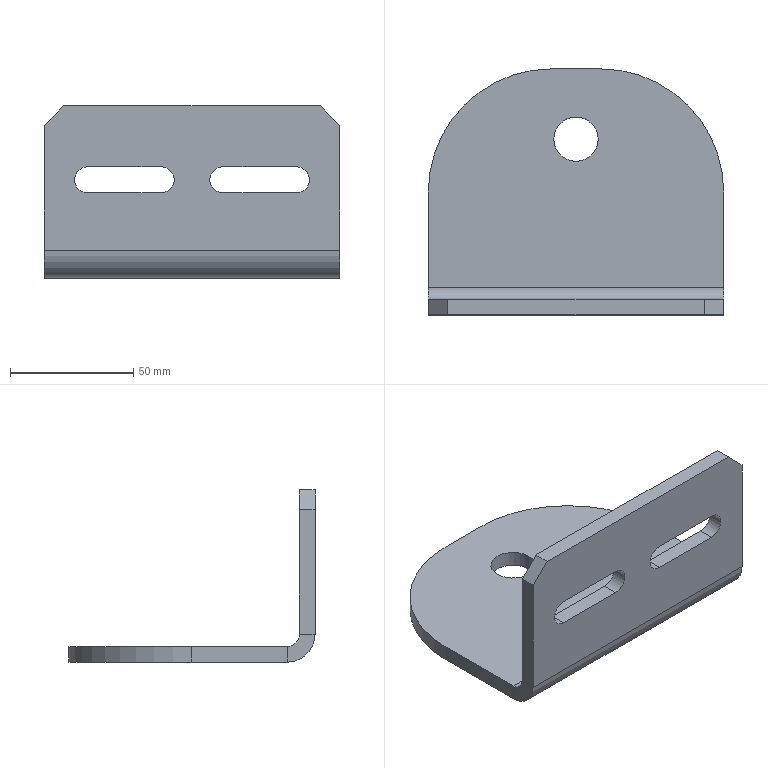Part | STEP file | BASE POLEA_SHEET METAL | 1 solid | 28 faces | box 120 x 100 x 70 mm | volume 108092 mm3 | plane 18 | cylinder 10 | commonest cylinder face diameters 10.5 x4 18 x2 100 x2 10 x1 22.7 x1
STEP:
#1=CARTESIAN_POINT('',(-9.,71.5,0.));
#2=VERTEX_POINT('',#1);
#3=CARTESIAN_POINT('',(9.,71.5,0.));
#4=VERTEX_POINT('',#3);
#5=CARTESIAN_POINT('',(0.,71.5,0.));
#6=DIRECTION('',(0.,0.,1.));
#7=DIRECTION('',(1.,0.,0.));
#8=AXIS2_PLACEMENT_3D('',#5,#6,#7);
#9=CIRCLE('',#8,9.);
#10=EDGE_CURVE('',#2,#4,#9,.T.);
#11=ORIENTED_EDGE('',*,*,#10,.F.);
#12=CARTESIAN_POINT('',(-9.,71.5,6.35));
#13=VERTEX_POINT('',#12);
#14=CARTESIAN_POINT('',(-9.,71.5,-3.65));
#15=DIRECTION('',(0.,0.,1.));
#16=VECTOR('',#15,1000.);
#17=LINE('',#14,#16);
#18=EDGE_CURVE('',#2,#13,#17,.T.);
#19=ORIENTED_EDGE('',*,*,#18,.T.);
#20=CARTESIAN_POINT('',(9.,71.5,6.35));
#21=VERTEX_POINT('',#20);
#22=CARTESIAN_POINT('',(0.,71.5,6.35));
#23=DIRECTION('',(0.,0.,1.));
#24=DIRECTION('',(1.,0.,0.));
#25=AXIS2_PLACEMENT_3D('',#22,#23,#24);
#26=CIRCLE('',#25,9.);
#27=EDGE_CURVE('',#13,#21,#26,.T.);
#28=ORIENTED_EDGE('',*,*,#27,.T.);
#29=CARTESIAN_POINT('',(9.,71.5,-3.65));
#30=DIRECTION('',(0.,0.,1.));
#31=VECTOR('',#30,1000.);
#32=LINE('',#29,#31);
#33=EDGE_CURVE('',#4,#21,#32,.T.);
#34=ORIENTED_EDGE('',*,*,#33,.F.);
#35=EDGE_LOOP('',(#11,#19,#28,#34));
#36=FACE_OUTER_BOUND('',#35,.T.);
#37=CARTESIAN_POINT('',(0.,71.5,-3.65));
#38=DIRECTION('',(0.,0.,1.));
#39=DIRECTION('',(1.,0.,0.));
#40=AXIS2_PLACEMENT_3D('',#37,#38,#39);
#41=CYLINDRICAL_SURFACE('',#40,9.);
#42=ADVANCED_FACE('',(#36),#41,.F.);
#43=CARTESIAN_POINT('',(60.,0.,11.35));
#44=VERTEX_POINT('',#43);
#45=CARTESIAN_POINT('',(60.,6.35,11.35));
#46=VERTEX_POINT('',#45);
#47=CARTESIAN_POINT('',(60.,0.,11.35));
#48=DIRECTION('',(0.,1.,0.));
#49=VECTOR('',#48,1000.);
#50=LINE('',#47,#49);
#51=EDGE_CURVE('',#44,#46,#50,.T.);
#52=ORIENTED_EDGE('',*,*,#51,.F.);
#53=CARTESIAN_POINT('',(60.,11.35,0.));
#54=VERTEX_POINT('',#53);
#55=CARTESIAN_POINT('',(60.,11.35,11.35));
#56=DIRECTION('',(1.,0.,0.));
#57=DIRECTION('',(0.,0.,1.));
#58=AXIS2_PLACEMENT_3D('',#55,#56,#57);
#59=CIRCLE('',#58,11.35);
#60=EDGE_CURVE('',#44,#54,#59,.T.);
#61=ORIENTED_EDGE('',*,*,#60,.T.);
#62=CARTESIAN_POINT('',(60.,11.35,6.35));
#63=VERTEX_POINT('',#62);
#64=CARTESIAN_POINT('',(60.,11.35,6.35));
#65=DIRECTION('',(0.,0.,-1.));
#66=VECTOR('',#65,1000.);
#67=LINE('',#64,#66);
#68=EDGE_CURVE('',#63,#54,#67,.T.);
#69=ORIENTED_EDGE('',*,*,#68,.F.);
#70=CARTESIAN_POINT('',(60.,11.35,11.35));
#71=DIRECTION('',(1.,0.,0.));
#72=DIRECTION('',(0.,0.,-1.));
#73=AXIS2_PLACEMENT_3D('',#70,#71,#72);
#74=CIRCLE('',#73,5.);
#75=EDGE_CURVE('',#46,#63,#74,.T.);
#76=ORIENTED_EDGE('',*,*,#75,.F.);
#77=EDGE_LOOP('',(#52,#61,#69,#76));
#78=FACE_OUTER_BOUND('',#77,.T.);
#79=CARTESIAN_POINT('',(60.,0.,11.35));
#80=DIRECTION('',(1.,0.,0.));
#81=DIRECTION('',(0.,0.,-1.));
#82=AXIS2_PLACEMENT_3D('',#79,#80,#81);
#83=PLANE('',#82);
#84=ADVANCED_FACE('',(#78),#83,.T.);
#85=CARTESIAN_POINT('',(60.,6.35,62.));
#86=VERTEX_POINT('',#85);
#87=CARTESIAN_POINT('',(60.,6.35,70.));
#88=DIRECTION('',(0.,0.,-1.));
#89=VECTOR('',#88,1000.);
#90=LINE('',#87,#89);
#91=EDGE_CURVE('',#86,#46,#90,.T.);
#92=ORIENTED_EDGE('',*,*,#91,.F.);
#93=CARTESIAN_POINT('',(60.,0.,62.));
#94=VERTEX_POINT('',#93);
#95=CARTESIAN_POINT('',(60.,11.35,62.));
#96=DIRECTION('',(0.,-1.,0.));
#97=VECTOR('',#96,1000.);
#98=LINE('',#95,#97);
#99=EDGE_CURVE('',#86,#94,#98,.T.);
#100=ORIENTED_EDGE('',*,*,#99,.T.);
#101=CARTESIAN_POINT('',(60.,0.,70.));
#102=DIRECTION('',(0.,0.,-1.));
#103=VECTOR('',#102,1000.);
#104=LINE('',#101,#103);
#105=EDGE_CURVE('',#94,#44,#104,.T.);
#106=ORIENTED_EDGE('',*,*,#105,.T.);
#107=ORIENTED_EDGE('',*,*,#51,.T.);
#108=EDGE_LOOP('',(#92,#100,#106,#107));
#109=FACE_OUTER_BOUND('',#108,.T.);
#110=CARTESIAN_POINT('',(60.,11.35,6.35));
#111=DIRECTION('',(1.,0.,0.));
#112=DIRECTION('',(0.,0.,-1.));
#113=AXIS2_PLACEMENT_3D('',#110,#111,#112);
#114=PLANE('',#113);
#115=ADVANCED_FACE('',(#109),#114,.T.);
#116=CARTESIAN_POINT('',(-60.,11.35,0.));
#117=VERTEX_POINT('',#116);
#118=CARTESIAN_POINT('',(-60.,11.35,6.35));
#119=VERTEX_POINT('',#118);
#120=CARTESIAN_POINT('',(-60.,11.35,0.));
#121=DIRECTION('',(0.,0.,1.));
#122=VECTOR('',#121,1000.);
#123=LINE('',#120,#122);
#124=EDGE_CURVE('',#117,#119,#123,.T.);
#125=ORIENTED_EDGE('',*,*,#124,.F.);
#126=CARTESIAN_POINT('',(-60.,0.,11.35));
#127=VERTEX_POINT('',#126);
#128=CARTESIAN_POINT('',(-60.,11.35,11.35));
#129=DIRECTION('',(1.,0.,0.));
#130=DIRECTION('',(0.,0.,1.));
#131=AXIS2_PLACEMENT_3D('',#128,#129,#130);
#132=CIRCLE('',#131,11.35);
#133=EDGE_CURVE('',#127,#117,#132,.T.);
#134=ORIENTED_EDGE('',*,*,#133,.F.);
#135=CARTESIAN_POINT('',(-60.,6.35,11.35));
#136=VERTEX_POINT('',#135);
#137=CARTESIAN_POINT('',(-60.,6.35,11.35));
#138=DIRECTION('',(0.,-1.,0.));
#139=VECTOR('',#138,1000.);
#140=LINE('',#137,#139);
#141=EDGE_CURVE('',#136,#127,#140,.T.);
#142=ORIENTED_EDGE('',*,*,#141,.F.);
#143=CARTESIAN_POINT('',(-60.,11.35,11.35));
#144=DIRECTION('',(1.,0.,0.));
#145=DIRECTION('',(0.,0.,-1.));
#146=AXIS2_PLACEMENT_3D('',#143,#144,#145);
#147=CIRCLE('',#146,5.);
#148=EDGE_CURVE('',#136,#119,#147,.T.);
#149=ORIENTED_EDGE('',*,*,#148,.T.);
#150=EDGE_LOOP('',(#125,#134,#142,#149));
#151=FACE_OUTER_BOUND('',#150,.T.);
#152=CARTESIAN_POINT('',(-60.,11.35,0.));
#153=DIRECTION('',(-1.,0.,0.));
#154=DIRECTION('',(0.,0.,1.));
#155=AXIS2_PLACEMENT_3D('',#152,#153,#154);
#156=PLANE('',#155);
#157=ADVANCED_FACE('',(#151),#156,.T.);
#158=CARTESIAN_POINT('',(-60.,50.,6.35));
#159=VERTEX_POINT('',#158);
#160=CARTESIAN_POINT('',(-60.,0.,6.35));
#161=DIRECTION('',(0.,1.,0.));
#162=VECTOR('',#161,1000.);
#163=LINE('',#160,#162);
#164=EDGE_CURVE('',#119,#159,#163,.T.);
#165=ORIENTED_EDGE('',*,*,#164,.T.);
#166=CARTESIAN_POINT('',(-60.,50.,0.));
#167=VERTEX_POINT('',#166);
#168=CARTESIAN_POINT('',(-60.,50.,11.35));
#169=DIRECTION('',(0.,0.,-1.));
#170=VECTOR('',#169,1000.);
#171=LINE('',#168,#170);
#172=EDGE_CURVE('',#159,#167,#171,.T.);
#173=ORIENTED_EDGE('',*,*,#172,.T.);
#174=CARTESIAN_POINT('',(-60.,0.,0.));
#175=DIRECTION('',(0.,1.,0.));
#176=VECTOR('',#175,1000.);
#177=LINE('',#174,#176);
#178=EDGE_CURVE('',#117,#167,#177,.T.);
#179=ORIENTED_EDGE('',*,*,#178,.F.);
#180=ORIENTED_EDGE('',*,*,#124,.T.);
#181=EDGE_LOOP('',(#165,#173,#179,#180));
#182=FACE_OUTER_BOUND('',#181,.T.);
#183=CARTESIAN_POINT('',(-60.,6.35,11.35));
#184=DIRECTION('',(-1.,0.,0.));
#185=DIRECTION('',(0.,0.,1.));
#186=AXIS2_PLACEMENT_3D('',#183,#184,#185);
#187=PLANE('',#186);
#188=ADVANCED_FACE('',(#182),#187,.T.);
#189=CARTESIAN_POINT('',(0.,71.5,0.));
#190=DIRECTION('',(0.,0.,1.));
#191=DIRECTION('',(1.,0.,0.));
#192=AXIS2_PLACEMENT_3D('',#189,#190,#191);
#193=CIRCLE('',#192,9.);
#194=EDGE_CURVE('',#4,#2,#193,.T.);
#195=ORIENTED_EDGE('',*,*,#194,.T.);
#196=ORIENTED_EDGE('',*,*,#10,.T.);
#197=EDGE_LOOP('',(#195,#196));
#198=FACE_BOUND('',#197,.T.);
#199=ORIENTED_EDGE('',*,*,#178,.T.);
#200=CARTESIAN_POINT('',(-10.,100.,0.));
#201=VERTEX_POINT('',#200);
#202=CARTESIAN_POINT('',(-10.,50.,0.));
#203=DIRECTION('',(0.,0.,-1.));
#204=DIRECTION('',(1.,0.,0.));
#205=AXIS2_PLACEMENT_3D('',#202,#203,#204);
#206=CIRCLE('',#205,50.);
#207=EDGE_CURVE('',#167,#201,#206,.T.);
#208=ORIENTED_EDGE('',*,*,#207,.T.);
#209=CARTESIAN_POINT('',(10.,100.,0.));
#210=VERTEX_POINT('',#209);
#211=CARTESIAN_POINT('',(60.,100.,0.));
#212=DIRECTION('',(-1.,0.,0.));
#213=VECTOR('',#212,1000.);
#214=LINE('',#211,#213);
#215=EDGE_CURVE('',#210,#201,#214,.T.);
#216=ORIENTED_EDGE('',*,*,#215,.F.);
#217=CARTESIAN_POINT('',(60.,50.,0.));
#218=VERTEX_POINT('',#217);
#219=CARTESIAN_POINT('',(10.,50.,0.));
#220=DIRECTION('',(0.,0.,-1.));
#221=DIRECTION('',(1.,0.,0.));
#222=AXIS2_PLACEMENT_3D('',#219,#220,#221);
#223=CIRCLE('',#222,50.);
#224=EDGE_CURVE('',#210,#218,#223,.T.);
#225=ORIENTED_EDGE('',*,*,#224,.T.);
#226=CARTESIAN_POINT('',(60.,0.,0.));
#227=DIRECTION('',(0.,1.,0.));
#228=VECTOR('',#227,1000.);
#229=LINE('',#226,#228);
#230=EDGE_CURVE('',#54,#218,#229,.T.);
#231=ORIENTED_EDGE('',*,*,#230,.F.);
#232=CARTESIAN_POINT('',(60.,11.35,0.));
#233=DIRECTION('',(-1.,0.,0.));
#234=VECTOR('',#233,1000.);
#235=LINE('',#232,#234);
#236=EDGE_CURVE('',#54,#117,#235,.T.);
#237=ORIENTED_EDGE('',*,*,#236,.T.);
#238=EDGE_LOOP('',(#199,#208,#216,#225,#231,#237));
#239=FACE_OUTER_BOUND('',#238,.T.);
#240=CARTESIAN_POINT('',(60.,0.,0.));
#241=DIRECTION('',(0.,0.,1.));
#242=DIRECTION('',(1.,0.,0.));
#243=AXIS2_PLACEMENT_3D('',#240,#241,#242);
#244=PLANE('',#243);
#245=ADVANCED_FACE('',(#198,#239),#244,.F.);
#246=ORIENTED_EDGE('',*,*,#215,.T.);
#247=CARTESIAN_POINT('',(-10.,100.,6.35));
#248=VERTEX_POINT('',#247);
#249=CARTESIAN_POINT('',(-10.,100.,6.35));
#250=DIRECTION('',(0.,0.,1.));
#251=VECTOR('',#250,1000.);
#252=LINE('',#249,#251);
#253=EDGE_CURVE('',#201,#248,#252,.T.);
#254=ORIENTED_EDGE('',*,*,#253,.T.);
#255=CARTESIAN_POINT('',(10.,100.,6.35));
#256=VERTEX_POINT('',#255);
#257=CARTESIAN_POINT('',(60.,100.,6.35));
#258=DIRECTION('',(-1.,0.,0.));
#259=VECTOR('',#258,1000.);
#260=LINE('',#257,#259);
#261=EDGE_CURVE('',#256,#248,#260,.T.);
#262=ORIENTED_EDGE('',*,*,#261,.F.);
#263=CARTESIAN_POINT('',(10.,100.,6.35));
#264=DIRECTION('',(0.,0.,-1.));
#265=VECTOR('',#264,1000.);
#266=LINE('',#263,#265);
#267=EDGE_CURVE('',#256,#210,#266,.T.);
#268=ORIENTED_EDGE('',*,*,#267,.T.);
#269=EDGE_LOOP('',(#246,#254,#262,#268));
#270=FACE_OUTER_BOUND('',#269,.T.);
#271=CARTESIAN_POINT('',(60.,100.,6.35));
#272=DIRECTION('',(0.,1.,0.));
#273=DIRECTION('',(0.,0.,1.));
#274=AXIS2_PLACEMENT_3D('',#271,#272,#273);
#275=PLANE('',#274);
#276=ADVANCED_FACE('',(#270),#275,.T.);
#277=CARTESIAN_POINT('',(0.,71.5,6.35));
#278=DIRECTION('',(0.,0.,1.));
#279=DIRECTION('',(1.,0.,0.));
#280=AXIS2_PLACEMENT_3D('',#277,#278,#279);
#281=CIRCLE('',#280,9.);
#282=EDGE_CURVE('',#21,#13,#281,.T.);
#283=ORIENTED_EDGE('',*,*,#282,.F.);
#284=ORIENTED_EDGE('',*,*,#27,.F.);
#285=EDGE_LOOP('',(#283,#284));
#286=FACE_BOUND('',#285,.T.);
#287=ORIENTED_EDGE('',*,*,#261,.T.);
#288=CARTESIAN_POINT('',(-10.,50.,6.35));
#289=DIRECTION('',(0.,0.,1.));
#290=DIRECTION('',(1.,0.,0.));
#291=AXIS2_PLACEMENT_3D('',#288,#289,#290);
#292=CIRCLE('',#291,50.);
#293=EDGE_CURVE('',#248,#159,#292,.T.);
#294=ORIENTED_EDGE('',*,*,#293,.T.);
#295=ORIENTED_EDGE('',*,*,#164,.F.);
#296=CARTESIAN_POINT('',(60.,11.35,6.35));
#297=DIRECTION('',(-1.,0.,0.));
#298=VECTOR('',#297,1000.);
#299=LINE('',#296,#298);
#300=EDGE_CURVE('',#63,#119,#299,.T.);
#301=ORIENTED_EDGE('',*,*,#300,.F.);
#302=CARTESIAN_POINT('',(60.,50.,6.35));
#303=VERTEX_POINT('',#302);
#304=CARTESIAN_POINT('',(60.,0.,6.35));
#305=DIRECTION('',(0.,1.,0.));
#306=VECTOR('',#305,1000.);
#307=LINE('',#304,#306);
#308=EDGE_CURVE('',#63,#303,#307,.T.);
#309=ORIENTED_EDGE('',*,*,#308,.T.);
#310=CARTESIAN_POINT('',(10.,50.,6.35));
#311=DIRECTION('',(0.,0.,1.));
#312=DIRECTION('',(1.,0.,0.));
#313=AXIS2_PLACEMENT_3D('',#310,#311,#312);
#314=CIRCLE('',#313,50.);
#315=EDGE_CURVE('',#303,#256,#314,.T.);
#316=ORIENTED_EDGE('',*,*,#315,.T.);
#317=EDGE_LOOP('',(#287,#294,#295,#301,#309,#316));
#318=FACE_OUTER_BOUND('',#317,.T.);
#319=CARTESIAN_POINT('',(60.,0.,6.35));
#320=DIRECTION('',(0.,0.,1.));
#321=DIRECTION('',(1.,0.,0.));
#322=AXIS2_PLACEMENT_3D('',#319,#320,#321);
#323=PLANE('',#322);
#324=ADVANCED_FACE('',(#286,#318),#323,.T.);
#325=ORIENTED_EDGE('',*,*,#148,.F.);
#326=CARTESIAN_POINT('',(60.,6.35,11.35));
#327=DIRECTION('',(-1.,0.,0.));
#328=VECTOR('',#327,1000.);
#329=LINE('',#326,#328);
#330=EDGE_CURVE('',#46,#136,#329,.T.);
#331=ORIENTED_EDGE('',*,*,#330,.F.);
#332=ORIENTED_EDGE('',*,*,#75,.T.);
#333=ORIENTED_EDGE('',*,*,#300,.T.);
#334=EDGE_LOOP('',(#325,#331,#332,#333));
#335=FACE_OUTER_BOUND('',#334,.T.);
#336=CARTESIAN_POINT('',(60.,11.35,11.35));
#337=DIRECTION('',(-1.,0.,0.));
#338=DIRECTION('',(0.,0.,1.));
#339=AXIS2_PLACEMENT_3D('',#336,#337,#338);
#340=CYLINDRICAL_SURFACE('',#339,5.);
#341=ADVANCED_FACE('',(#335),#340,.F.);
#342=CARTESIAN_POINT('',(-42.5,6.35,34.75));
#343=VERTEX_POINT('',#342);
#344=CARTESIAN_POINT('',(-42.5,6.35,45.25));
#345=VERTEX_POINT('',#344);
#346=CARTESIAN_POINT('',(-42.5,6.35,40.));
#347=DIRECTION('',(0.,1.,0.));
#348=DIRECTION('',(0.,0.,1.));
#349=AXIS2_PLACEMENT_3D('',#346,#347,#348);
#350=CIRCLE('',#349,5.25);
#351=EDGE_CURVE('',#343,#345,#350,.T.);
#352=ORIENTED_EDGE('',*,*,#351,.F.);
#353=CARTESIAN_POINT('',(-12.5,6.35,34.75));
#354=VERTEX_POINT('',#353);
#355=CARTESIAN_POINT('',(-42.5,6.35,34.75));
#356=DIRECTION('',(-1.,0.,0.));
#357=VECTOR('',#356,1000.);
#358=LINE('',#355,#357);
#359=EDGE_CURVE('',#354,#343,#358,.T.);
#360=ORIENTED_EDGE('',*,*,#359,.F.);
#361=CARTESIAN_POINT('',(-12.5,6.35,45.25));
#362=VERTEX_POINT('',#361);
#363=CARTESIAN_POINT('',(-12.5,6.35,40.));
#364=DIRECTION('',(0.,1.,0.));
#365=DIRECTION('',(0.,0.,1.));
#366=AXIS2_PLACEMENT_3D('',#363,#364,#365);
#367=CIRCLE('',#366,5.25);
#368=EDGE_CURVE('',#362,#354,#367,.T.);
#369=ORIENTED_EDGE('',*,*,#368,.F.);
#370=CARTESIAN_POINT('',(-42.5,6.35,45.25));
#371=DIRECTION('',(1.,0.,0.));
#372=VECTOR('',#371,1000.);
#373=LINE('',#370,#372);
#374=EDGE_CURVE('',#345,#362,#373,.T.);
#375=ORIENTED_EDGE('',*,*,#374,.F.);
#376=EDGE_LOOP('',(#352,#360,#369,#375));
#377=FACE_BOUND('',#376,.T.);
#378=CARTESIAN_POINT('',(42.5,6.35,45.25));
#379=VERTEX_POINT('',#378);
#380=CARTESIAN_POINT('',(42.5,6.35,34.75));
#381=VERTEX_POINT('',#380);
#382=CARTESIAN_POINT('',(42.5,6.35,40.));
#383=DIRECTION('',(0.,1.,0.));
#384=DIRECTION('',(0.,0.,-1.));
#385=AXIS2_PLACEMENT_3D('',#382,#383,#384);
#386=CIRCLE('',#385,5.25);
#387=EDGE_CURVE('',#379,#381,#386,.T.);
#388=ORIENTED_EDGE('',*,*,#387,.F.);
#389=CARTESIAN_POINT('',(12.5,6.35,45.25));
#390=VERTEX_POINT('',#389);
#391=CARTESIAN_POINT('',(42.5,6.35,45.25));
#392=DIRECTION('',(1.,0.,0.));
#393=VECTOR('',#392,1000.);
#394=LINE('',#391,#393);
#395=EDGE_CURVE('',#390,#379,#394,.T.);
#396=ORIENTED_EDGE('',*,*,#395,.F.);
#397=CARTESIAN_POINT('',(12.5,6.35,34.75));
#398=VERTEX_POINT('',#397);
#399=CARTESIAN_POINT('',(12.5,6.35,40.));
#400=DIRECTION('',(0.,1.,0.));
#401=DIRECTION('',(0.,0.,-1.));
#402=AXIS2_PLACEMENT_3D('',#399,#400,#401);
#403=CIRCLE('',#402,5.25);
#404=EDGE_CURVE('',#398,#390,#403,.T.);
#405=ORIENTED_EDGE('',*,*,#404,.F.);
#406=CARTESIAN_POINT('',(42.5,6.35,34.75));
#407=DIRECTION('',(-1.,0.,0.));
#408=VECTOR('',#407,1000.);
#409=LINE('',#406,#408);
#410=EDGE_CURVE('',#381,#398,#409,.T.);
#411=ORIENTED_EDGE('',*,*,#410,.F.);
#412=EDGE_LOOP('',(#388,#396,#405,#411));
#413=FACE_BOUND('',#412,.T.);
#414=CARTESIAN_POINT('',(-60.,6.35,62.));
#415=VERTEX_POINT('',#414);
#416=CARTESIAN_POINT('',(-60.,6.35,70.));
#417=DIRECTION('',(0.,0.,-1.));
#418=VECTOR('',#417,1000.);
#419=LINE('',#416,#418);
#420=EDGE_CURVE('',#415,#136,#419,.T.);
#421=ORIENTED_EDGE('',*,*,#420,.F.);
#422=CARTESIAN_POINT('',(-52.,6.35,70.));
#423=VERTEX_POINT('',#422);
#424=CARTESIAN_POINT('',(4.,6.35,126.));
#425=DIRECTION('',(0.7071,0.,0.7071));
#426=VECTOR('',#425,1000.);
#427=LINE('',#424,#426);
#428=EDGE_CURVE('',#415,#423,#427,.T.);
#429=ORIENTED_EDGE('',*,*,#428,.T.);
#430=CARTESIAN_POINT('',(52.,6.35,70.));
#431=VERTEX_POINT('',#430);
#432=CARTESIAN_POINT('',(60.,6.35,70.));
#433=DIRECTION('',(-1.,0.,0.));
#434=VECTOR('',#433,1000.);
#435=LINE('',#432,#434);
#436=EDGE_CURVE('',#431,#423,#435,.T.);
#437=ORIENTED_EDGE('',*,*,#436,.F.);
#438=CARTESIAN_POINT('',(56.,6.35,66.));
#439=DIRECTION('',(0.7071,0.,-0.7071));
#440=VECTOR('',#439,1000.);
#441=LINE('',#438,#440);
#442=EDGE_CURVE('',#431,#86,#441,.T.);
#443=ORIENTED_EDGE('',*,*,#442,.T.);
#444=ORIENTED_EDGE('',*,*,#91,.T.);
#445=ORIENTED_EDGE('',*,*,#330,.T.);
#446=EDGE_LOOP('',(#421,#429,#437,#443,#444,#445));
#447=FACE_OUTER_BOUND('',#446,.T.);
#448=CARTESIAN_POINT('',(60.,6.35,70.));
#449=DIRECTION('',(0.,1.,0.));
#450=DIRECTION('',(0.,0.,1.));
#451=AXIS2_PLACEMENT_3D('',#448,#449,#450);
#452=PLANE('',#451);
#453=ADVANCED_FACE('',(#377,#413,#447),#452,.T.);
#454=ORIENTED_EDGE('',*,*,#436,.T.);
#455=CARTESIAN_POINT('',(-52.,0.,70.));
#456=VERTEX_POINT('',#455);
#457=CARTESIAN_POINT('',(-52.,0.,70.));
#458=DIRECTION('',(0.,-1.,0.));
#459=VECTOR('',#458,1000.);
#460=LINE('',#457,#459);
#461=EDGE_CURVE('',#423,#456,#460,.T.);
#462=ORIENTED_EDGE('',*,*,#461,.T.);
#463=CARTESIAN_POINT('',(52.,0.,70.));
#464=VERTEX_POINT('',#463);
#465=CARTESIAN_POINT('',(60.,0.,70.));
#466=DIRECTION('',(-1.,0.,0.));
#467=VECTOR('',#466,1000.);
#468=LINE('',#465,#467);
#469=EDGE_CURVE('',#464,#456,#468,.T.);
#470=ORIENTED_EDGE('',*,*,#469,.F.);
#471=CARTESIAN_POINT('',(52.,0.,70.));
#472=DIRECTION('',(0.,1.,0.));
#473=VECTOR('',#472,1000.);
#474=LINE('',#471,#473);
#475=EDGE_CURVE('',#464,#431,#474,.T.);
#476=ORIENTED_EDGE('',*,*,#475,.T.);
#477=EDGE_LOOP('',(#454,#462,#470,#476));
#478=FACE_OUTER_BOUND('',#477,.T.);
#479=CARTESIAN_POINT('',(60.,0.,70.));
#480=DIRECTION('',(0.,0.,1.));
#481=DIRECTION('',(1.,0.,0.));
#482=AXIS2_PLACEMENT_3D('',#479,#480,#481);
#483=PLANE('',#482);
#484=ADVANCED_FACE('',(#478),#483,.T.);
#485=CARTESIAN_POINT('',(-12.5,0.,34.75));
#486=VERTEX_POINT('',#485);
#487=CARTESIAN_POINT('',(-42.5,0.,34.75));
#488=VERTEX_POINT('',#487);
#489=CARTESIAN_POINT('',(-42.5,0.,34.75));
#490=DIRECTION('',(-1.,0.,0.));
#491=VECTOR('',#490,1000.);
#492=LINE('',#489,#491);
#493=EDGE_CURVE('',#486,#488,#492,.T.);
#494=ORIENTED_EDGE('',*,*,#493,.T.);
#495=CARTESIAN_POINT('',(-42.5,0.,45.25));
#496=VERTEX_POINT('',#495);
#497=CARTESIAN_POINT('',(-42.5,0.,40.));
#498=DIRECTION('',(0.,1.,0.));
#499=DIRECTION('',(0.,0.,1.));
#500=AXIS2_PLACEMENT_3D('',#497,#498,#499);
#501=CIRCLE('',#500,5.25);
#502=EDGE_CURVE('',#488,#496,#501,.T.);
#503=ORIENTED_EDGE('',*,*,#502,.T.);
#504=CARTESIAN_POINT('',(-12.5,0.,45.25));
#505=VERTEX_POINT('',#504);
#506=CARTESIAN_POINT('',(-42.5,0.,45.25));
#507=DIRECTION('',(1.,0.,0.));
#508=VECTOR('',#507,1000.);
#509=LINE('',#506,#508);
#510=EDGE_CURVE('',#496,#505,#509,.T.);
#511=ORIENTED_EDGE('',*,*,#510,.T.);
#512=CARTESIAN_POINT('',(-12.5,0.,40.));
#513=DIRECTION('',(0.,1.,0.));
#514=DIRECTION('',(0.,0.,1.));
#515=AXIS2_PLACEMENT_3D('',#512,#513,#514);
#516=CIRCLE('',#515,5.25);
#517=EDGE_CURVE('',#505,#486,#516,.T.);
#518=ORIENTED_EDGE('',*,*,#517,.T.);
#519=EDGE_LOOP('',(#494,#503,#511,#518));
#520=FACE_BOUND('',#519,.T.);
#521=CARTESIAN_POINT('',(12.5,0.,45.25));
#522=VERTEX_POINT('',#521);
#523=CARTESIAN_POINT('',(42.5,0.,45.25));
#524=VERTEX_POINT('',#523);
#525=CARTESIAN_POINT('',(42.5,0.,45.25));
#526=DIRECTION('',(1.,0.,0.));
#527=VECTOR('',#526,1000.);
#528=LINE('',#525,#527);
#529=EDGE_CURVE('',#522,#524,#528,.T.);
#530=ORIENTED_EDGE('',*,*,#529,.T.);
#531=CARTESIAN_POINT('',(42.5,0.,34.75));
#532=VERTEX_POINT('',#531);
#533=CARTESIAN_POINT('',(42.5,0.,40.));
#534=DIRECTION('',(0.,1.,0.));
#535=DIRECTION('',(0.,0.,-1.));
#536=AXIS2_PLACEMENT_3D('',#533,#534,#535);
#537=CIRCLE('',#536,5.25);
#538=EDGE_CURVE('',#524,#532,#537,.T.);
#539=ORIENTED_EDGE('',*,*,#538,.T.);
#540=CARTESIAN_POINT('',(12.5,0.,34.75));
#541=VERTEX_POINT('',#540);
#542=CARTESIAN_POINT('',(42.5,0.,34.75));
#543=DIRECTION('',(-1.,0.,0.));
#544=VECTOR('',#543,1000.);
#545=LINE('',#542,#544);
#546=EDGE_CURVE('',#532,#541,#545,.T.);
#547=ORIENTED_EDGE('',*,*,#546,.T.);
#548=CARTESIAN_POINT('',(12.5,0.,40.));
#549=DIRECTION('',(0.,1.,0.));
#550=DIRECTION('',(0.,0.,-1.));
#551=AXIS2_PLACEMENT_3D('',#548,#549,#550);
#552=CIRCLE('',#551,5.25);
#553=EDGE_CURVE('',#541,#522,#552,.T.);
#554=ORIENTED_EDGE('',*,*,#553,.T.);
#555=EDGE_LOOP('',(#530,#539,#547,#554));
#556=FACE_BOUND('',#555,.T.);
#557=ORIENTED_EDGE('',*,*,#469,.T.);
#558=CARTESIAN_POINT('',(-60.,0.,62.));
#559=VERTEX_POINT('',#558);
#560=CARTESIAN_POINT('',(-60.,0.,62.));
#561=DIRECTION('',(-0.7071,0.,-0.7071));
#562=VECTOR('',#561,1000.);
#563=LINE('',#560,#562);
#564=EDGE_CURVE('',#456,#559,#563,.T.);
#565=ORIENTED_EDGE('',*,*,#564,.T.);
#566=CARTESIAN_POINT('',(-60.,0.,70.));
#567=DIRECTION('',(0.,0.,-1.));
#568=VECTOR('',#567,1000.);
#569=LINE('',#566,#568);
#570=EDGE_CURVE('',#559,#127,#569,.T.);
#571=ORIENTED_EDGE('',*,*,#570,.T.);
#572=CARTESIAN_POINT('',(60.,0.,11.35));
#573=DIRECTION('',(-1.,0.,0.));
#574=VECTOR('',#573,1000.);
#575=LINE('',#572,#574);
#576=EDGE_CURVE('',#44,#127,#575,.T.);
#577=ORIENTED_EDGE('',*,*,#576,.F.);
#578=ORIENTED_EDGE('',*,*,#105,.F.);
#579=CARTESIAN_POINT('',(52.,0.,70.));
#580=DIRECTION('',(-0.7071,0.,0.7071));
#581=VECTOR('',#580,1000.);
#582=LINE('',#579,#581);
#583=EDGE_CURVE('',#94,#464,#582,.T.);
#584=ORIENTED_EDGE('',*,*,#583,.T.);
#585=EDGE_LOOP('',(#557,#565,#571,#577,#578,#584));
#586=FACE_OUTER_BOUND('',#585,.T.);
#587=CARTESIAN_POINT('',(60.,0.,70.));
#588=DIRECTION('',(0.,1.,0.));
#589=DIRECTION('',(0.,0.,1.));
#590=AXIS2_PLACEMENT_3D('',#587,#588,#589);
#591=PLANE('',#590);
#592=ADVANCED_FACE('',(#520,#556,#586),#591,.F.);
#593=ORIENTED_EDGE('',*,*,#133,.T.);
#594=ORIENTED_EDGE('',*,*,#236,.F.);
#595=ORIENTED_EDGE('',*,*,#60,.F.);
#596=ORIENTED_EDGE('',*,*,#576,.T.);
#597=EDGE_LOOP('',(#593,#594,#595,#596));
#598=FACE_OUTER_BOUND('',#597,.T.);
#599=CARTESIAN_POINT('',(60.,11.35,11.35));
#600=DIRECTION('',(-1.,0.,0.));
#601=DIRECTION('',(0.,0.,1.));
#602=AXIS2_PLACEMENT_3D('',#599,#600,#601);
#603=CYLINDRICAL_SURFACE('',#602,11.35);
#604=ADVANCED_FACE('',(#598),#603,.T.);
#605=ORIENTED_EDGE('',*,*,#230,.T.);
#606=CARTESIAN_POINT('',(60.,50.,11.35));
#607=DIRECTION('',(0.,0.,1.));
#608=VECTOR('',#607,1000.);
#609=LINE('',#606,#608);
#610=EDGE_CURVE('',#218,#303,#609,.T.);
#611=ORIENTED_EDGE('',*,*,#610,.T.);
#612=ORIENTED_EDGE('',*,*,#308,.F.);
#613=ORIENTED_EDGE('',*,*,#68,.T.);
#614=EDGE_LOOP('',(#605,#611,#612,#613));
#615=FACE_OUTER_BOUND('',#614,.T.);
#616=CARTESIAN_POINT('',(60.,11.35,11.35));
#617=DIRECTION('',(1.,0.,0.));
#618=DIRECTION('',(0.,0.,-1.));
#619=AXIS2_PLACEMENT_3D('',#616,#617,#618);
#620=PLANE('',#619);
#621=ADVANCED_FACE('',(#615),#620,.T.);
#622=ORIENTED_EDGE('',*,*,#570,.F.);
#623=CARTESIAN_POINT('',(-60.,6.35,62.));
#624=DIRECTION('',(0.,1.,0.));
#625=VECTOR('',#624,1000.);
#626=LINE('',#623,#625);
#627=EDGE_CURVE('',#559,#415,#626,.T.);
#628=ORIENTED_EDGE('',*,*,#627,.T.);
#629=ORIENTED_EDGE('',*,*,#420,.T.);
#630=ORIENTED_EDGE('',*,*,#141,.T.);
#631=EDGE_LOOP('',(#622,#628,#629,#630));
#632=FACE_OUTER_BOUND('',#631,.T.);
#633=CARTESIAN_POINT('',(-60.,11.35,11.35));
#634=DIRECTION('',(1.,0.,0.));
#635=DIRECTION('',(0.,0.,-1.));
#636=AXIS2_PLACEMENT_3D('',#633,#634,#635);
#637=PLANE('',#636);
#638=ADVANCED_FACE('',(#632),#637,.F.);
#639=ORIENTED_EDGE('',*,*,#18,.F.);
#640=ORIENTED_EDGE('',*,*,#194,.F.);
#641=ORIENTED_EDGE('',*,*,#33,.T.);
#642=ORIENTED_EDGE('',*,*,#282,.T.);
#643=EDGE_LOOP('',(#639,#640,#641,#642));
#644=FACE_OUTER_BOUND('',#643,.T.);
#645=CARTESIAN_POINT('',(0.,71.5,-3.65));
#646=DIRECTION('',(0.,0.,1.));
#647=DIRECTION('',(1.,0.,0.));
#648=AXIS2_PLACEMENT_3D('',#645,#646,#647);
#649=CYLINDRICAL_SURFACE('',#648,9.);
#650=ADVANCED_FACE('',(#644),#649,.F.);
#651=ORIENTED_EDGE('',*,*,#293,.F.);
#652=ORIENTED_EDGE('',*,*,#253,.F.);
#653=ORIENTED_EDGE('',*,*,#207,.F.);
#654=ORIENTED_EDGE('',*,*,#172,.F.);
#655=EDGE_LOOP('',(#651,#652,#653,#654));
#656=FACE_OUTER_BOUND('',#655,.T.);
#657=CARTESIAN_POINT('',(-10.,50.,11.35));
#658=DIRECTION('',(0.,0.,-1.));
#659=DIRECTION('',(-1.,0.,0.));
#660=AXIS2_PLACEMENT_3D('',#657,#658,#659);
#661=CYLINDRICAL_SURFACE('',#660,50.);
#662=ADVANCED_FACE('',(#656),#661,.T.);
#663=ORIENTED_EDGE('',*,*,#315,.F.);
#664=ORIENTED_EDGE('',*,*,#610,.F.);
#665=ORIENTED_EDGE('',*,*,#224,.F.);
#666=ORIENTED_EDGE('',*,*,#267,.F.);
#667=EDGE_LOOP('',(#663,#664,#665,#666));
#668=FACE_OUTER_BOUND('',#667,.T.);
#669=CARTESIAN_POINT('',(10.,50.,6.35));
#670=DIRECTION('',(0.,0.,-1.));
#671=DIRECTION('',(-1.,0.,0.));
#672=AXIS2_PLACEMENT_3D('',#669,#670,#671);
#673=CYLINDRICAL_SURFACE('',#672,50.);
#674=ADVANCED_FACE('',(#668),#673,.T.);
#675=ORIENTED_EDGE('',*,*,#564,.F.);
#676=ORIENTED_EDGE('',*,*,#461,.F.);
#677=ORIENTED_EDGE('',*,*,#428,.F.);
#678=ORIENTED_EDGE('',*,*,#627,.F.);
#679=EDGE_LOOP('',(#675,#676,#677,#678));
#680=FACE_OUTER_BOUND('',#679,.T.);
#681=CARTESIAN_POINT('',(-60.,11.35,62.));
#682=DIRECTION('',(-0.7071,0.,0.7071));
#683=DIRECTION('',(0.,-1.,0.));
#684=AXIS2_PLACEMENT_3D('',#681,#682,#683);
#685=PLANE('',#684);
#686=ADVANCED_FACE('',(#680),#685,.T.);
#687=ORIENTED_EDGE('',*,*,#583,.F.);
#688=ORIENTED_EDGE('',*,*,#99,.F.);
#689=ORIENTED_EDGE('',*,*,#442,.F.);
#690=ORIENTED_EDGE('',*,*,#475,.F.);
#691=EDGE_LOOP('',(#687,#688,#689,#690));
#692=FACE_OUTER_BOUND('',#691,.T.);
#693=CARTESIAN_POINT('',(52.,0.,70.));
#694=DIRECTION('',(-0.7071,0.,-0.7071));
#695=DIRECTION('',(0.,1.,0.));
#696=AXIS2_PLACEMENT_3D('',#693,#694,#695);
#697=PLANE('',#696);
#698=ADVANCED_FACE('',(#692),#697,.F.);
#699=ORIENTED_EDGE('',*,*,#387,.T.);
#700=CARTESIAN_POINT('',(42.5,0.,34.75));
#701=DIRECTION('',(0.,1.,0.));
#702=VECTOR('',#701,1000.);
#703=LINE('',#700,#702);
#704=EDGE_CURVE('',#532,#381,#703,.T.);
#705=ORIENTED_EDGE('',*,*,#704,.F.);
#706=ORIENTED_EDGE('',*,*,#538,.F.);
#707=CARTESIAN_POINT('',(42.5,0.,45.25));
#708=DIRECTION('',(0.,1.,0.));
#709=VECTOR('',#708,1000.);
#710=LINE('',#707,#709);
#711=EDGE_CURVE('',#524,#379,#710,.T.);
#712=ORIENTED_EDGE('',*,*,#711,.T.);
#713=EDGE_LOOP('',(#699,#705,#706,#712));
#714=FACE_OUTER_BOUND('',#713,.T.);
#715=CARTESIAN_POINT('',(42.5,0.,40.));
#716=DIRECTION('',(0.,1.,0.));
#717=DIRECTION('',(0.,0.,1.));
#718=AXIS2_PLACEMENT_3D('',#715,#716,#717);
#719=CYLINDRICAL_SURFACE('',#718,5.25);
#720=ADVANCED_FACE('',(#714),#719,.F.);
#721=ORIENTED_EDGE('',*,*,#395,.T.);
#722=ORIENTED_EDGE('',*,*,#711,.F.);
#723=ORIENTED_EDGE('',*,*,#529,.F.);
#724=CARTESIAN_POINT('',(12.5,0.,45.25));
#725=DIRECTION('',(0.,1.,0.));
#726=VECTOR('',#725,1000.);
#727=LINE('',#724,#726);
#728=EDGE_CURVE('',#522,#390,#727,.T.);
#729=ORIENTED_EDGE('',*,*,#728,.T.);
#730=EDGE_LOOP('',(#721,#722,#723,#729));
#731=FACE_OUTER_BOUND('',#730,.T.);
#732=CARTESIAN_POINT('',(42.5,0.,45.25));
#733=DIRECTION('',(0.,0.,1.));
#734=DIRECTION('',(1.,0.,0.));
#735=AXIS2_PLACEMENT_3D('',#732,#733,#734);
#736=PLANE('',#735);
#737=ADVANCED_FACE('',(#731),#736,.F.);
#738=ORIENTED_EDGE('',*,*,#404,.T.);
#739=ORIENTED_EDGE('',*,*,#728,.F.);
#740=ORIENTED_EDGE('',*,*,#553,.F.);
#741=CARTESIAN_POINT('',(12.5,0.,34.75));
#742=DIRECTION('',(0.,1.,0.));
#743=VECTOR('',#742,1000.);
#744=LINE('',#741,#743);
#745=EDGE_CURVE('',#541,#398,#744,.T.);
#746=ORIENTED_EDGE('',*,*,#745,.T.);
#747=EDGE_LOOP('',(#738,#739,#740,#746));
#748=FACE_OUTER_BOUND('',#747,.T.);
#749=CARTESIAN_POINT('',(12.5,0.,40.));
#750=DIRECTION('',(0.,1.,0.));
#751=DIRECTION('',(0.,0.,1.));
#752=AXIS2_PLACEMENT_3D('',#749,#750,#751);
#753=CYLINDRICAL_SURFACE('',#752,5.25);
#754=ADVANCED_FACE('',(#748),#753,.F.);
#755=ORIENTED_EDGE('',*,*,#410,.T.);
#756=ORIENTED_EDGE('',*,*,#745,.F.);
#757=ORIENTED_EDGE('',*,*,#546,.F.);
#758=ORIENTED_EDGE('',*,*,#704,.T.);
#759=EDGE_LOOP('',(#755,#756,#757,#758));
#760=FACE_OUTER_BOUND('',#759,.T.);
#761=CARTESIAN_POINT('',(42.5,0.,34.75));
#762=DIRECTION('',(0.,0.,-1.));
#763=DIRECTION('',(-1.,0.,0.));
#764=AXIS2_PLACEMENT_3D('',#761,#762,#763);
#765=PLANE('',#764);
#766=ADVANCED_FACE('',(#760),#765,.F.);
#767=ORIENTED_EDGE('',*,*,#351,.T.);
#768=CARTESIAN_POINT('',(-42.5,0.,45.25));
#769=DIRECTION('',(0.,1.,0.));
#770=VECTOR('',#769,1000.);
#771=LINE('',#768,#770);
#772=EDGE_CURVE('',#496,#345,#771,.T.);
#773=ORIENTED_EDGE('',*,*,#772,.F.);
#774=ORIENTED_EDGE('',*,*,#502,.F.);
#775=CARTESIAN_POINT('',(-42.5,0.,34.75));
#776=DIRECTION('',(0.,1.,0.));
#777=VECTOR('',#776,1000.);
#778=LINE('',#775,#777);
#779=EDGE_CURVE('',#488,#343,#778,.T.);
#780=ORIENTED_EDGE('',*,*,#779,.T.);
#781=EDGE_LOOP('',(#767,#773,#774,#780));
#782=FACE_OUTER_BOUND('',#781,.T.);
#783=CARTESIAN_POINT('',(-42.5,0.,40.));
#784=DIRECTION('',(0.,1.,0.));
#785=DIRECTION('',(0.,0.,1.));
#786=AXIS2_PLACEMENT_3D('',#783,#784,#785);
#787=CYLINDRICAL_SURFACE('',#786,5.25);
#788=ADVANCED_FACE('',(#782),#787,.F.);
#789=ORIENTED_EDGE('',*,*,#359,.T.);
#790=ORIENTED_EDGE('',*,*,#779,.F.);
#791=ORIENTED_EDGE('',*,*,#493,.F.);
#792=CARTESIAN_POINT('',(-12.5,0.,34.75));
#793=DIRECTION('',(0.,1.,0.));
#794=VECTOR('',#793,1000.);
#795=LINE('',#792,#794);
#796=EDGE_CURVE('',#486,#354,#795,.T.);
#797=ORIENTED_EDGE('',*,*,#796,.T.);
#798=EDGE_LOOP('',(#789,#790,#791,#797));
#799=FACE_OUTER_BOUND('',#798,.T.);
#800=CARTESIAN_POINT('',(-42.5,0.,34.75));
#801=DIRECTION('',(0.,0.,-1.));
#802=DIRECTION('',(-1.,0.,0.));
#803=AXIS2_PLACEMENT_3D('',#800,#801,#802);
#804=PLANE('',#803);
#805=ADVANCED_FACE('',(#799),#804,.F.);
#806=ORIENTED_EDGE('',*,*,#368,.T.);
#807=ORIENTED_EDGE('',*,*,#796,.F.);
#808=ORIENTED_EDGE('',*,*,#517,.F.);
#809=CARTESIAN_POINT('',(-12.5,0.,45.25));
#810=DIRECTION('',(0.,1.,0.));
#811=VECTOR('',#810,1000.);
#812=LINE('',#809,#811);
#813=EDGE_CURVE('',#505,#362,#812,.T.);
#814=ORIENTED_EDGE('',*,*,#813,.T.);
#815=EDGE_LOOP('',(#806,#807,#808,#814));
#816=FACE_OUTER_BOUND('',#815,.T.);
#817=CARTESIAN_POINT('',(-12.5,0.,40.));
#818=DIRECTION('',(0.,1.,0.));
#819=DIRECTION('',(0.,0.,1.));
#820=AXIS2_PLACEMENT_3D('',#817,#818,#819);
#821=CYLINDRICAL_SURFACE('',#820,5.25);
#822=ADVANCED_FACE('',(#816),#821,.F.);
#823=ORIENTED_EDGE('',*,*,#374,.T.);
#824=ORIENTED_EDGE('',*,*,#813,.F.);
#825=ORIENTED_EDGE('',*,*,#510,.F.);
#826=ORIENTED_EDGE('',*,*,#772,.T.);
#827=EDGE_LOOP('',(#823,#824,#825,#826));
#828=FACE_OUTER_BOUND('',#827,.T.);
#829=CARTESIAN_POINT('',(-42.5,0.,45.25));
#830=DIRECTION('',(0.,0.,1.));
#831=DIRECTION('',(1.,0.,0.));
#832=AXIS2_PLACEMENT_3D('',#829,#830,#831);
#833=PLANE('',#832);
#834=ADVANCED_FACE('',(#828),#833,.F.);
#835=CLOSED_SHELL('',(#42,#84,#115,#157,#188,#245,#276,#324,#341,#453,#484,#592,#604,#621,#638,#650,#662,#674,#686,#698,#720,#737,#754,#766,#788,#805,#822,#834));
#836=MANIFOLD_SOLID_BREP('',#835);
#837=CARTESIAN_POINT('',(0.,0.,0.));
#838=DIRECTION('',(0.,0.,1.));
#839=DIRECTION('',(1.,0.,0.));
#840=AXIS2_PLACEMENT_3D('',#837,#838,#839);
#841=(LENGTH_UNIT()NAMED_UNIT(*)SI_UNIT(.MILLI.,.METRE.));
#842=UNCERTAINTY_MEASURE_WITH_UNIT(LENGTH_MEASURE(0.00001),#841,'','');
#843=(NAMED_UNIT(*)PLANE_ANGLE_UNIT()SI_UNIT($,.RADIAN.));
#844=(NAMED_UNIT(*)SI_UNIT($,.STERADIAN.)SOLID_ANGLE_UNIT());
#845=(GEOMETRIC_REPRESENTATION_CONTEXT(3)GLOBAL_UNCERTAINTY_ASSIGNED_CONTEXT((#842))GLOBAL_UNIT_ASSIGNED_CONTEXT((#841,#843,#844))REPRESENTATION_CONTEXT('',''));
#846=ADVANCED_BREP_SHAPE_REPRESENTATION('',(#836,#840),#845);